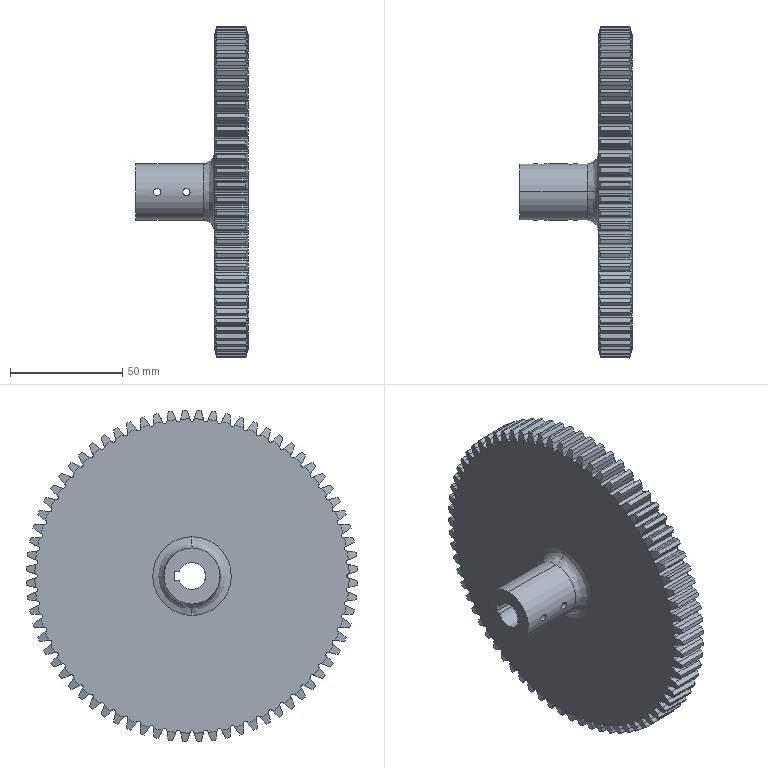Part | STEP file | 06-28 Gear 2-72 | 1 solid | 625 faces | box 50 x 147.929 x 147.929 mm | volume 253016 mm3 | plane 294 | cylinder 185 | cone 144 | spline 2 | commonest cylinder face diameters 2 x101 148 x72 3.3 x8 12 x2 25 x2